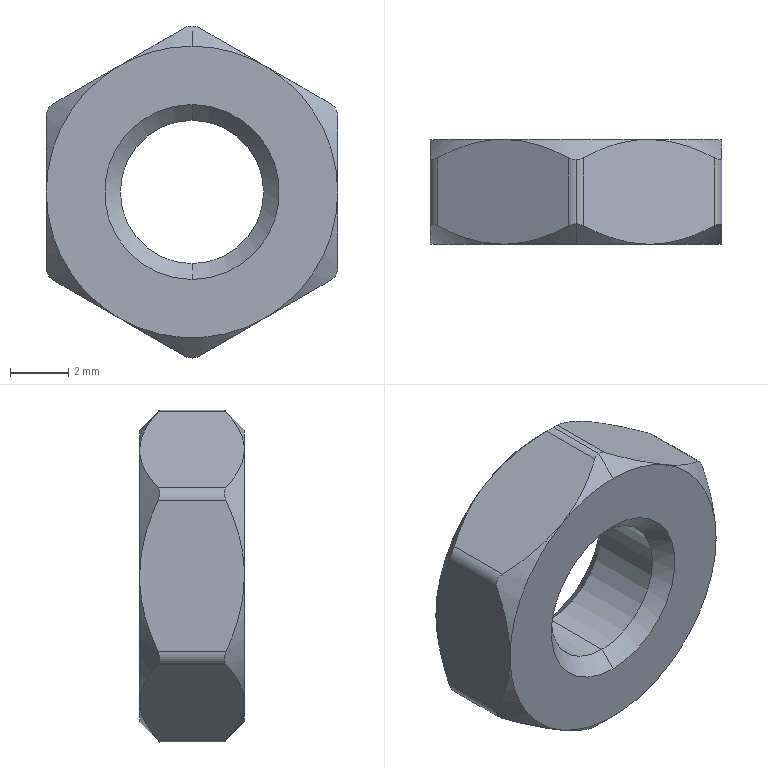Part | STEP file | _TDB86-M6-L20-002 | 1 solid | 35 faces | box 10 x 3.6 x 11.392 mm | volume 234.612 mm3 | cone 18 | cylinder 9 | plane 8 | commonest cylinder face diameters 1 x7 4.917 x2